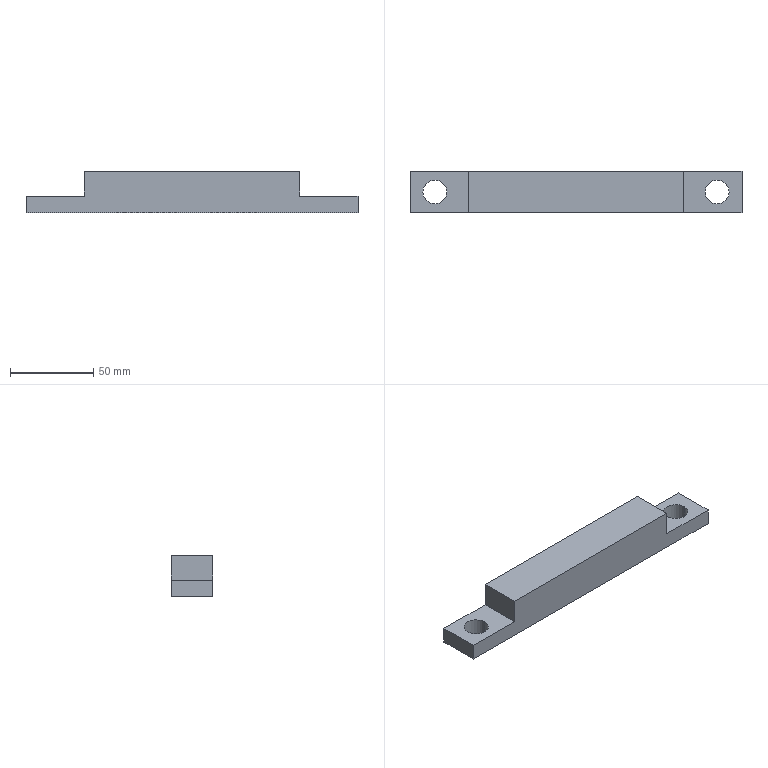Part | STEP file | 1 solid | 14 faces | box 200 x 25 x 25 mm | volume 95447 mm3 | plane 10 | cylinder 4 | commonest cylinder face diameters 14.5 x4
STEP:
#1=CARTESIAN_POINT('',(0.,0.,0.));
#2=DIRECTION('',(0.,0.,1.));
#3=DIRECTION('',(1.,0.,0.));
#4=AXIS2_PLACEMENT_3D('',#1,#2,#3);
#5=CARTESIAN_POINT('',(92.25,0.,0.));
#6=VERTEX_POINT('',#5);
#7=CARTESIAN_POINT('',(92.25,0.,10.));
#8=VERTEX_POINT('',#7);
#9=CARTESIAN_POINT('',(92.25,0.,-15.));
#10=DIRECTION('',(0.,0.,1.));
#11=VECTOR('',#10,1.);
#12=LINE('',#9,#11);
#13=CARTESIAN_POINT('',(85.,0.,-15.));
#14=DIRECTION('',(0.,0.,1.));
#15=DIRECTION('',(1.,0.,0.));
#16=AXIS2_PLACEMENT_3D('',#13,#14,#15);
#17=CYLINDRICAL_SURFACE('',#16,7.25);
#18=CARTESIAN_POINT('',(6.283,0.));
#19=DIRECTION('',(0.,1.));
#20=VECTOR('',#19,1.);
#21=LINE('',#18,#20);
#22=(GEOMETRIC_REPRESENTATION_CONTEXT(2)PARAMETRIC_REPRESENTATION_CONTEXT()REPRESENTATION_CONTEXT('',''));
#23=DEFINITIONAL_REPRESENTATION('',(#21),#22);
#24=PCURVE('',#17,#23);
#25=CARTESIAN_POINT('',(85.,0.,-15.));
#26=DIRECTION('',(0.,0.,1.));
#27=DIRECTION('',(1.,0.,0.));
#28=AXIS2_PLACEMENT_3D('',#25,#26,#27);
#29=CYLINDRICAL_SURFACE('',#28,7.25);
#30=CARTESIAN_POINT('',(0.,0.));
#31=DIRECTION('',(0.,1.));
#32=VECTOR('',#31,1.);
#33=LINE('',#30,#32);
#34=(GEOMETRIC_REPRESENTATION_CONTEXT(2)PARAMETRIC_REPRESENTATION_CONTEXT()REPRESENTATION_CONTEXT('',''));
#35=DEFINITIONAL_REPRESENTATION('',(#33),#34);
#36=PCURVE('',#29,#35);
#37=SURFACE_CURVE('',#12,(#24,#36),.PCURVE_S1.);
#38=EDGE_CURVE('',#6,#8,#37,.T.);
#39=ORIENTED_EDGE('',*,*,#38,.T.);
#40=CARTESIAN_POINT('',(77.75,0.,10.));
#41=VERTEX_POINT('',#40);
#42=CARTESIAN_POINT('',(85.,0.,10.));
#43=DIRECTION('',(0.,0.,1.));
#44=DIRECTION('',(1.,0.,0.));
#45=AXIS2_PLACEMENT_3D('',#42,#43,#44);
#46=CIRCLE('',#45,7.25);
#47=CARTESIAN_POINT('',(0.,25.));
#48=DIRECTION('',(1.,0.));
#49=VECTOR('',#48,1.);
#50=LINE('',#47,#49);
#51=(GEOMETRIC_REPRESENTATION_CONTEXT(2)PARAMETRIC_REPRESENTATION_CONTEXT()REPRESENTATION_CONTEXT('',''));
#52=DEFINITIONAL_REPRESENTATION('',(#50),#51);
#53=PCURVE('',#17,#52);
#54=CARTESIAN_POINT('',(100.,-12.5,10.));
#55=DIRECTION('',(0.,0.,-1.));
#56=DIRECTION('',(-1.,0.,0.));
#57=AXIS2_PLACEMENT_3D('',#54,#55,#56);
#58=PLANE('',#57);
#59=CARTESIAN_POINT('',(7.75,12.5));
#60=CARTESIAN_POINT('',(7.75,25.057));
#61=CARTESIAN_POINT('',(18.625,18.779));
#62=CARTESIAN_POINT('',(29.5,12.5));
#63=CARTESIAN_POINT('',(18.625,6.221));
#64=CARTESIAN_POINT('',(7.75,-0.05737));
#65=CARTESIAN_POINT('',(7.75,12.5));
#66=(BOUNDED_CURVE()B_SPLINE_CURVE(2,(#59,#60,#61,#62,#63,#64,#65),.UNSPECIFIED.,.T.,.F.)B_SPLINE_CURVE_WITH_KNOTS((1,2,2,2,2,1),(-2.094,0.,2.094,4.189,6.283,8.378),.UNSPECIFIED.)CURVE()GEOMETRIC_REPRESENTATION_ITEM()RATIONAL_B_SPLINE_CURVE((1.,0.5,1.,0.5,1.,0.5,1.))REPRESENTATION_ITEM(''));
#67=(GEOMETRIC_REPRESENTATION_CONTEXT(2)PARAMETRIC_REPRESENTATION_CONTEXT()REPRESENTATION_CONTEXT('',''));
#68=DEFINITIONAL_REPRESENTATION('',(#66),#67);
#69=PCURVE('',#58,#68);
#70=SURFACE_CURVE('',#46,(#53,#69),.PCURVE_S1.);
#71=EDGE_CURVE('',#41,#8,#70,.T.);
#72=ORIENTED_EDGE('',*,*,#71,.F.);
#73=CARTESIAN_POINT('',(77.75,0.,0.));
#74=VERTEX_POINT('',#73);
#75=CARTESIAN_POINT('',(77.75,0.,-15.));
#76=DIRECTION('',(0.,0.,1.));
#77=VECTOR('',#76,1.);
#78=LINE('',#75,#77);
#79=CARTESIAN_POINT('',(3.142,0.));
#80=DIRECTION('',(0.,1.));
#81=VECTOR('',#80,1.);
#82=LINE('',#79,#81);
#83=(GEOMETRIC_REPRESENTATION_CONTEXT(2)PARAMETRIC_REPRESENTATION_CONTEXT()REPRESENTATION_CONTEXT('',''));
#84=DEFINITIONAL_REPRESENTATION('',(#82),#83);
#85=PCURVE('',#17,#84);
#86=CARTESIAN_POINT('',(3.142,0.));
#87=DIRECTION('',(0.,1.));
#88=VECTOR('',#87,1.);
#89=LINE('',#86,#88);
#90=(GEOMETRIC_REPRESENTATION_CONTEXT(2)PARAMETRIC_REPRESENTATION_CONTEXT()REPRESENTATION_CONTEXT('',''));
#91=DEFINITIONAL_REPRESENTATION('',(#89),#90);
#92=PCURVE('',#29,#91);
#93=SURFACE_CURVE('',#78,(#85,#92),.PCURVE_S1.);
#94=EDGE_CURVE('',#74,#41,#93,.T.);
#95=ORIENTED_EDGE('',*,*,#94,.F.);
#96=CARTESIAN_POINT('',(85.,0.,0.));
#97=DIRECTION('',(0.,0.,-1.));
#98=DIRECTION('',(-1.,0.,0.));
#99=AXIS2_PLACEMENT_3D('',#96,#97,#98);
#100=CIRCLE('',#99,7.25);
#101=CARTESIAN_POINT('',(9.425,15.));
#102=DIRECTION('',(-1.,0.));
#103=VECTOR('',#102,1.);
#104=LINE('',#101,#103);
#105=(GEOMETRIC_REPRESENTATION_CONTEXT(2)PARAMETRIC_REPRESENTATION_CONTEXT()REPRESENTATION_CONTEXT('',''));
#106=DEFINITIONAL_REPRESENTATION('',(#104),#105);
#107=PCURVE('',#17,#106);
#108=CARTESIAN_POINT('',(0.,0.,0.));
#109=DIRECTION('',(0.,0.,-1.));
#110=DIRECTION('',(-1.,0.,0.));
#111=AXIS2_PLACEMENT_3D('',#108,#109,#110);
#112=PLANE('',#111);
#113=CARTESIAN_POINT('',(-85.,0.));
#114=DIRECTION('',(1.,0.));
#115=AXIS2_PLACEMENT_2D('',#113,#114);
#116=CIRCLE('',#115,7.25);
#117=(GEOMETRIC_REPRESENTATION_CONTEXT(2)PARAMETRIC_REPRESENTATION_CONTEXT()REPRESENTATION_CONTEXT('',''));
#118=DEFINITIONAL_REPRESENTATION('',(#116),#117);
#119=PCURVE('',#112,#118);
#120=SURFACE_CURVE('',#100,(#107,#119),.PCURVE_S1.);
#121=EDGE_CURVE('',#6,#74,#120,.T.);
#122=ORIENTED_EDGE('',*,*,#121,.F.);
#123=EDGE_LOOP('',(#39,#72,#95,#122));
#124=FACE_BOUND('',#123,.F.);
#125=ADVANCED_FACE('',(#124),#17,.F.);
#126=CARTESIAN_POINT('',(-77.75,0.,0.));
#127=VERTEX_POINT('',#126);
#128=CARTESIAN_POINT('',(-77.75,0.,10.));
#129=VERTEX_POINT('',#128);
#130=CARTESIAN_POINT('',(-77.75,0.,-15.));
#131=DIRECTION('',(0.,0.,1.));
#132=VECTOR('',#131,1.);
#133=LINE('',#130,#132);
#134=CARTESIAN_POINT('',(-85.,0.,-15.));
#135=DIRECTION('',(0.,0.,1.));
#136=DIRECTION('',(1.,0.,0.));
#137=AXIS2_PLACEMENT_3D('',#134,#135,#136);
#138=CYLINDRICAL_SURFACE('',#137,7.25);
#139=CARTESIAN_POINT('',(6.283,0.));
#140=DIRECTION('',(0.,1.));
#141=VECTOR('',#140,1.);
#142=LINE('',#139,#141);
#143=(GEOMETRIC_REPRESENTATION_CONTEXT(2)PARAMETRIC_REPRESENTATION_CONTEXT()REPRESENTATION_CONTEXT('',''));
#144=DEFINITIONAL_REPRESENTATION('',(#142),#143);
#145=PCURVE('',#138,#144);
#146=CARTESIAN_POINT('',(-85.,0.,-15.));
#147=DIRECTION('',(0.,0.,1.));
#148=DIRECTION('',(1.,0.,0.));
#149=AXIS2_PLACEMENT_3D('',#146,#147,#148);
#150=CYLINDRICAL_SURFACE('',#149,7.25);
#151=CARTESIAN_POINT('',(0.,0.));
#152=DIRECTION('',(0.,1.));
#153=VECTOR('',#152,1.);
#154=LINE('',#151,#153);
#155=(GEOMETRIC_REPRESENTATION_CONTEXT(2)PARAMETRIC_REPRESENTATION_CONTEXT()REPRESENTATION_CONTEXT('',''));
#156=DEFINITIONAL_REPRESENTATION('',(#154),#155);
#157=PCURVE('',#150,#156);
#158=SURFACE_CURVE('',#133,(#145,#157),.PCURVE_S1.);
#159=EDGE_CURVE('',#127,#129,#158,.T.);
#160=ORIENTED_EDGE('',*,*,#159,.T.);
#161=CARTESIAN_POINT('',(-92.25,0.,10.));
#162=VERTEX_POINT('',#161);
#163=CARTESIAN_POINT('',(-85.,0.,10.));
#164=DIRECTION('',(0.,0.,1.));
#165=DIRECTION('',(1.,0.,0.));
#166=AXIS2_PLACEMENT_3D('',#163,#164,#165);
#167=CIRCLE('',#166,7.25);
#168=CARTESIAN_POINT('',(0.,25.));
#169=DIRECTION('',(1.,0.));
#170=VECTOR('',#169,1.);
#171=LINE('',#168,#170);
#172=(GEOMETRIC_REPRESENTATION_CONTEXT(2)PARAMETRIC_REPRESENTATION_CONTEXT()REPRESENTATION_CONTEXT('',''));
#173=DEFINITIONAL_REPRESENTATION('',(#171),#172);
#174=PCURVE('',#138,#173);
#175=CARTESIAN_POINT('',(-100.,-12.5,10.));
#176=DIRECTION('',(0.,0.,-1.));
#177=DIRECTION('',(-1.,0.,0.));
#178=AXIS2_PLACEMENT_3D('',#175,#176,#177);
#179=PLANE('',#178);
#180=CARTESIAN_POINT('',(-22.25,12.5));
#181=CARTESIAN_POINT('',(-22.25,25.057));
#182=CARTESIAN_POINT('',(-11.375,18.779));
#183=CARTESIAN_POINT('',(-0.5,12.5));
#184=CARTESIAN_POINT('',(-11.375,6.221));
#185=CARTESIAN_POINT('',(-22.25,-0.05737));
#186=CARTESIAN_POINT('',(-22.25,12.5));
#187=(BOUNDED_CURVE()B_SPLINE_CURVE(2,(#180,#181,#182,#183,#184,#185,#186),.UNSPECIFIED.,.T.,.F.)B_SPLINE_CURVE_WITH_KNOTS((1,2,2,2,2,1),(-2.094,0.,2.094,4.189,6.283,8.378),.UNSPECIFIED.)CURVE()GEOMETRIC_REPRESENTATION_ITEM()RATIONAL_B_SPLINE_CURVE((1.,0.5,1.,0.5,1.,0.5,1.))REPRESENTATION_ITEM(''));
#188=(GEOMETRIC_REPRESENTATION_CONTEXT(2)PARAMETRIC_REPRESENTATION_CONTEXT()REPRESENTATION_CONTEXT('',''));
#189=DEFINITIONAL_REPRESENTATION('',(#187),#188);
#190=PCURVE('',#179,#189);
#191=SURFACE_CURVE('',#167,(#174,#190),.PCURVE_S1.);
#192=EDGE_CURVE('',#162,#129,#191,.T.);
#193=ORIENTED_EDGE('',*,*,#192,.F.);
#194=CARTESIAN_POINT('',(-92.25,0.,0.));
#195=VERTEX_POINT('',#194);
#196=CARTESIAN_POINT('',(-92.25,0.,-15.));
#197=DIRECTION('',(0.,0.,1.));
#198=VECTOR('',#197,1.);
#199=LINE('',#196,#198);
#200=CARTESIAN_POINT('',(3.142,0.));
#201=DIRECTION('',(0.,1.));
#202=VECTOR('',#201,1.);
#203=LINE('',#200,#202);
#204=(GEOMETRIC_REPRESENTATION_CONTEXT(2)PARAMETRIC_REPRESENTATION_CONTEXT()REPRESENTATION_CONTEXT('',''));
#205=DEFINITIONAL_REPRESENTATION('',(#203),#204);
#206=PCURVE('',#138,#205);
#207=CARTESIAN_POINT('',(3.142,0.));
#208=DIRECTION('',(0.,1.));
#209=VECTOR('',#208,1.);
#210=LINE('',#207,#209);
#211=(GEOMETRIC_REPRESENTATION_CONTEXT(2)PARAMETRIC_REPRESENTATION_CONTEXT()REPRESENTATION_CONTEXT('',''));
#212=DEFINITIONAL_REPRESENTATION('',(#210),#211);
#213=PCURVE('',#150,#212);
#214=SURFACE_CURVE('',#199,(#206,#213),.PCURVE_S1.);
#215=EDGE_CURVE('',#195,#162,#214,.T.);
#216=ORIENTED_EDGE('',*,*,#215,.F.);
#217=CARTESIAN_POINT('',(-85.,0.,0.));
#218=DIRECTION('',(0.,0.,-1.));
#219=DIRECTION('',(-1.,0.,0.));
#220=AXIS2_PLACEMENT_3D('',#217,#218,#219);
#221=CIRCLE('',#220,7.25);
#222=CARTESIAN_POINT('',(9.425,15.));
#223=DIRECTION('',(-1.,0.));
#224=VECTOR('',#223,1.);
#225=LINE('',#222,#224);
#226=(GEOMETRIC_REPRESENTATION_CONTEXT(2)PARAMETRIC_REPRESENTATION_CONTEXT()REPRESENTATION_CONTEXT('',''));
#227=DEFINITIONAL_REPRESENTATION('',(#225),#226);
#228=PCURVE('',#138,#227);
#229=CARTESIAN_POINT('',(85.,0.));
#230=DIRECTION('',(1.,0.));
#231=AXIS2_PLACEMENT_2D('',#229,#230);
#232=CIRCLE('',#231,7.25);
#233=(GEOMETRIC_REPRESENTATION_CONTEXT(2)PARAMETRIC_REPRESENTATION_CONTEXT()REPRESENTATION_CONTEXT('',''));
#234=DEFINITIONAL_REPRESENTATION('',(#232),#233);
#235=PCURVE('',#112,#234);
#236=SURFACE_CURVE('',#221,(#228,#235),.PCURVE_S1.);
#237=EDGE_CURVE('',#127,#195,#236,.T.);
#238=ORIENTED_EDGE('',*,*,#237,.F.);
#239=EDGE_LOOP('',(#160,#193,#216,#238));
#240=FACE_BOUND('',#239,.F.);
#241=ADVANCED_FACE('',(#240),#138,.F.);
#242=CARTESIAN_POINT('',(-100.,-12.5,10.));
#243=VERTEX_POINT('',#242);
#244=CARTESIAN_POINT('',(-100.,-12.5,0.));
#245=VERTEX_POINT('',#244);
#246=CARTESIAN_POINT('',(-100.,-12.5,25.));
#247=DIRECTION('',(0.,0.,-1.));
#248=VECTOR('',#247,1.);
#249=LINE('',#246,#248);
#250=CARTESIAN_POINT('',(-100.,12.5,25.));
#251=DIRECTION('',(1.,0.,0.));
#252=DIRECTION('',(0.,0.,-1.));
#253=AXIS2_PLACEMENT_3D('',#250,#251,#252);
#254=PLANE('',#253);
#255=CARTESIAN_POINT('',(0.,-25.));
#256=DIRECTION('',(1.,0.));
#257=VECTOR('',#256,1.);
#258=LINE('',#255,#257);
#259=(GEOMETRIC_REPRESENTATION_CONTEXT(2)PARAMETRIC_REPRESENTATION_CONTEXT()REPRESENTATION_CONTEXT('',''));
#260=DEFINITIONAL_REPRESENTATION('',(#258),#259);
#261=PCURVE('',#254,#260);
#262=CARTESIAN_POINT('',(100.,-12.5,25.));
#263=DIRECTION('',(0.,1.,0.));
#264=DIRECTION('',(-1.,0.,0.));
#265=AXIS2_PLACEMENT_3D('',#262,#263,#264);
#266=PLANE('',#265);
#267=CARTESIAN_POINT('',(200.,0.));
#268=DIRECTION('',(0.,-1.));
#269=VECTOR('',#268,1.);
#270=LINE('',#267,#269);
#271=(GEOMETRIC_REPRESENTATION_CONTEXT(2)PARAMETRIC_REPRESENTATION_CONTEXT()REPRESENTATION_CONTEXT('',''));
#272=DEFINITIONAL_REPRESENTATION('',(#270),#271);
#273=PCURVE('',#266,#272);
#274=SURFACE_CURVE('',#249,(#261,#273),.PCURVE_S1.);
#275=EDGE_CURVE('',#243,#245,#274,.T.);
#276=ORIENTED_EDGE('',*,*,#275,.F.);
#277=CARTESIAN_POINT('',(-100.,12.5,10.));
#278=VERTEX_POINT('',#277);
#279=CARTESIAN_POINT('',(-100.,-12.5,10.));
#280=DIRECTION('',(0.,1.,0.));
#281=VECTOR('',#280,1.);
#282=LINE('',#279,#281);
#283=CARTESIAN_POINT('',(15.,-25.));
#284=DIRECTION('',(0.,1.));
#285=VECTOR('',#284,1.);
#286=LINE('',#283,#285);
#287=(GEOMETRIC_REPRESENTATION_CONTEXT(2)PARAMETRIC_REPRESENTATION_CONTEXT()REPRESENTATION_CONTEXT('',''));
#288=DEFINITIONAL_REPRESENTATION('',(#286),#287);
#289=PCURVE('',#254,#288);
#290=CARTESIAN_POINT('',(0.,0.));
#291=DIRECTION('',(0.,1.));
#292=VECTOR('',#291,1.);
#293=LINE('',#290,#292);
#294=(GEOMETRIC_REPRESENTATION_CONTEXT(2)PARAMETRIC_REPRESENTATION_CONTEXT()REPRESENTATION_CONTEXT('',''));
#295=DEFINITIONAL_REPRESENTATION('',(#293),#294);
#296=PCURVE('',#179,#295);
#297=SURFACE_CURVE('',#282,(#289,#296),.PCURVE_S1.);
#298=EDGE_CURVE('',#243,#278,#297,.T.);
#299=ORIENTED_EDGE('',*,*,#298,.T.);
#300=CARTESIAN_POINT('',(-100.,12.5,0.));
#301=VERTEX_POINT('',#300);
#302=CARTESIAN_POINT('',(-100.,12.5,25.));
#303=DIRECTION('',(0.,0.,-1.));
#304=VECTOR('',#303,1.);
#305=LINE('',#302,#304);
#306=CARTESIAN_POINT('',(0.,0.));
#307=DIRECTION('',(1.,0.));
#308=VECTOR('',#307,1.);
#309=LINE('',#306,#308);
#310=(GEOMETRIC_REPRESENTATION_CONTEXT(2)PARAMETRIC_REPRESENTATION_CONTEXT()REPRESENTATION_CONTEXT('',''));
#311=DEFINITIONAL_REPRESENTATION('',(#309),#310);
#312=PCURVE('',#254,#311);
#313=CARTESIAN_POINT('',(100.,12.5,25.));
#314=DIRECTION('',(0.,-1.,0.));
#315=DIRECTION('',(1.,0.,0.));
#316=AXIS2_PLACEMENT_3D('',#313,#314,#315);
#317=PLANE('',#316);
#318=CARTESIAN_POINT('',(-200.,0.));
#319=DIRECTION('',(0.,-1.));
#320=VECTOR('',#319,1.);
#321=LINE('',#318,#320);
#322=(GEOMETRIC_REPRESENTATION_CONTEXT(2)PARAMETRIC_REPRESENTATION_CONTEXT()REPRESENTATION_CONTEXT('',''));
#323=DEFINITIONAL_REPRESENTATION('',(#321),#322);
#324=PCURVE('',#317,#323);
#325=SURFACE_CURVE('',#305,(#312,#324),.PCURVE_S1.);
#326=EDGE_CURVE('',#278,#301,#325,.T.);
#327=ORIENTED_EDGE('',*,*,#326,.T.);
#328=CARTESIAN_POINT('',(-100.,12.5,0.));
#329=DIRECTION('',(0.,-1.,0.));
#330=VECTOR('',#329,1.);
#331=LINE('',#328,#330);
#332=CARTESIAN_POINT('',(25.,0.));
#333=DIRECTION('',(0.,-1.));
#334=VECTOR('',#333,1.);
#335=LINE('',#332,#334);
#336=(GEOMETRIC_REPRESENTATION_CONTEXT(2)PARAMETRIC_REPRESENTATION_CONTEXT()REPRESENTATION_CONTEXT('',''));
#337=DEFINITIONAL_REPRESENTATION('',(#335),#336);
#338=PCURVE('',#254,#337);
#339=CARTESIAN_POINT('',(100.,12.5));
#340=DIRECTION('',(0.,-1.));
#341=VECTOR('',#340,1.);
#342=LINE('',#339,#341);
#343=(GEOMETRIC_REPRESENTATION_CONTEXT(2)PARAMETRIC_REPRESENTATION_CONTEXT()REPRESENTATION_CONTEXT('',''));
#344=DEFINITIONAL_REPRESENTATION('',(#342),#343);
#345=PCURVE('',#112,#344);
#346=SURFACE_CURVE('',#331,(#338,#345),.PCURVE_S1.);
#347=EDGE_CURVE('',#301,#245,#346,.T.);
#348=ORIENTED_EDGE('',*,*,#347,.T.);
#349=EDGE_LOOP('',(#276,#299,#327,#348));
#350=FACE_BOUND('',#349,.T.);
#351=ADVANCED_FACE('',(#350),#254,.F.);
#352=CARTESIAN_POINT('',(-65.,-12.5,25.));
#353=VERTEX_POINT('',#352);
#354=CARTESIAN_POINT('',(-65.,-12.5,10.));
#355=VERTEX_POINT('',#354);
#356=CARTESIAN_POINT('',(-65.,-12.5,10.));
#357=DIRECTION('',(0.,0.,-1.));
#358=VECTOR('',#357,1.);
#359=LINE('',#356,#358);
#360=CARTESIAN_POINT('',(165.,-15.));
#361=DIRECTION('',(0.,-1.));
#362=VECTOR('',#361,1.);
#363=LINE('',#360,#362);
#364=(GEOMETRIC_REPRESENTATION_CONTEXT(2)PARAMETRIC_REPRESENTATION_CONTEXT()REPRESENTATION_CONTEXT('',''));
#365=DEFINITIONAL_REPRESENTATION('',(#363),#364);
#366=PCURVE('',#266,#365);
#367=CARTESIAN_POINT('',(-65.,-12.5,10.));
#368=DIRECTION('',(1.,0.,0.));
#369=DIRECTION('',(0.,1.,0.));
#370=AXIS2_PLACEMENT_3D('',#367,#368,#369);
#371=PLANE('',#370);
#372=CARTESIAN_POINT('',(0.,0.));
#373=DIRECTION('',(0.,-1.));
#374=VECTOR('',#373,1.);
#375=LINE('',#372,#374);
#376=(GEOMETRIC_REPRESENTATION_CONTEXT(2)PARAMETRIC_REPRESENTATION_CONTEXT()REPRESENTATION_CONTEXT('',''));
#377=DEFINITIONAL_REPRESENTATION('',(#375),#376);
#378=PCURVE('',#371,#377);
#379=SURFACE_CURVE('',#359,(#366,#378),.PCURVE_S1.);
#380=EDGE_CURVE('',#353,#355,#379,.T.);
#381=ORIENTED_EDGE('',*,*,#380,.T.);
#382=CARTESIAN_POINT('',(-100.,-12.5,10.));
#383=DIRECTION('',(-1.,0.,0.));
#384=VECTOR('',#383,1.);
#385=LINE('',#382,#384);
#386=CARTESIAN_POINT('',(200.,-15.));
#387=DIRECTION('',(1.,0.));
#388=VECTOR('',#387,1.);
#389=LINE('',#386,#388);
#390=(GEOMETRIC_REPRESENTATION_CONTEXT(2)PARAMETRIC_REPRESENTATION_CONTEXT()REPRESENTATION_CONTEXT('',''));
#391=DEFINITIONAL_REPRESENTATION('',(#389),#390);
#392=PCURVE('',#266,#391);
#393=CARTESIAN_POINT('',(0.,0.));
#394=DIRECTION('',(1.,0.));
#395=VECTOR('',#394,1.);
#396=LINE('',#393,#395);
#397=(GEOMETRIC_REPRESENTATION_CONTEXT(2)PARAMETRIC_REPRESENTATION_CONTEXT()REPRESENTATION_CONTEXT('',''));
#398=DEFINITIONAL_REPRESENTATION('',(#396),#397);
#399=PCURVE('',#179,#398);
#400=SURFACE_CURVE('',#385,(#392,#399),.PCURVE_S1.);
#401=EDGE_CURVE('',#355,#243,#400,.T.);
#402=ORIENTED_EDGE('',*,*,#401,.T.);
#403=ORIENTED_EDGE('',*,*,#275,.T.);
#404=CARTESIAN_POINT('',(100.,-12.5,0.));
#405=VERTEX_POINT('',#404);
#406=CARTESIAN_POINT('',(100.,-12.5,0.));
#407=DIRECTION('',(1.,0.,0.));
#408=VECTOR('',#407,1.);
#409=LINE('',#406,#408);
#410=CARTESIAN_POINT('',(0.,-25.));
#411=DIRECTION('',(-1.,0.));
#412=VECTOR('',#411,1.);
#413=LINE('',#410,#412);
#414=(GEOMETRIC_REPRESENTATION_CONTEXT(2)PARAMETRIC_REPRESENTATION_CONTEXT()REPRESENTATION_CONTEXT('',''));
#415=DEFINITIONAL_REPRESENTATION('',(#413),#414);
#416=PCURVE('',#266,#415);
#417=CARTESIAN_POINT('',(-100.,-12.5));
#418=DIRECTION('',(-1.,0.));
#419=VECTOR('',#418,1.);
#420=LINE('',#417,#419);
#421=(GEOMETRIC_REPRESENTATION_CONTEXT(2)PARAMETRIC_REPRESENTATION_CONTEXT()REPRESENTATION_CONTEXT('',''));
#422=DEFINITIONAL_REPRESENTATION('',(#420),#421);
#423=PCURVE('',#112,#422);
#424=SURFACE_CURVE('',#409,(#416,#423),.PCURVE_S1.);
#425=EDGE_CURVE('',#245,#405,#424,.T.);
#426=ORIENTED_EDGE('',*,*,#425,.T.);
#427=CARTESIAN_POINT('',(100.,-12.5,10.));
#428=VERTEX_POINT('',#427);
#429=CARTESIAN_POINT('',(100.,-12.5,25.));
#430=DIRECTION('',(0.,0.,-1.));
#431=VECTOR('',#430,1.);
#432=LINE('',#429,#431);
#433=CARTESIAN_POINT('',(0.,0.));
#434=DIRECTION('',(0.,-1.));
#435=VECTOR('',#434,1.);
#436=LINE('',#433,#435);
#437=(GEOMETRIC_REPRESENTATION_CONTEXT(2)PARAMETRIC_REPRESENTATION_CONTEXT()REPRESENTATION_CONTEXT('',''));
#438=DEFINITIONAL_REPRESENTATION('',(#436),#437);
#439=PCURVE('',#266,#438);
#440=CARTESIAN_POINT('',(100.,12.5,25.));
#441=DIRECTION('',(-1.,0.,0.));
#442=DIRECTION('',(0.,0.,1.));
#443=AXIS2_PLACEMENT_3D('',#440,#441,#442);
#444=PLANE('',#443);
#445=CARTESIAN_POINT('',(0.,-25.));
#446=DIRECTION('',(-1.,0.));
#447=VECTOR('',#446,1.);
#448=LINE('',#445,#447);
#449=(GEOMETRIC_REPRESENTATION_CONTEXT(2)PARAMETRIC_REPRESENTATION_CONTEXT()REPRESENTATION_CONTEXT('',''));
#450=DEFINITIONAL_REPRESENTATION('',(#448),#449);
#451=PCURVE('',#444,#450);
#452=SURFACE_CURVE('',#432,(#439,#451),.PCURVE_S1.);
#453=EDGE_CURVE('',#428,#405,#452,.T.);
#454=ORIENTED_EDGE('',*,*,#453,.F.);
#455=CARTESIAN_POINT('',(65.,-12.5,10.));
#456=VERTEX_POINT('',#455);
#457=CARTESIAN_POINT('',(100.,-12.5,10.));
#458=DIRECTION('',(-1.,0.,0.));
#459=VECTOR('',#458,1.);
#460=LINE('',#457,#459);
#461=CARTESIAN_POINT('',(0.,-15.));
#462=DIRECTION('',(1.,0.));
#463=VECTOR('',#462,1.);
#464=LINE('',#461,#463);
#465=(GEOMETRIC_REPRESENTATION_CONTEXT(2)PARAMETRIC_REPRESENTATION_CONTEXT()REPRESENTATION_CONTEXT('',''));
#466=DEFINITIONAL_REPRESENTATION('',(#464),#465);
#467=PCURVE('',#266,#466);
#468=CARTESIAN_POINT('',(0.,0.));
#469=DIRECTION('',(1.,0.));
#470=VECTOR('',#469,1.);
#471=LINE('',#468,#470);
#472=(GEOMETRIC_REPRESENTATION_CONTEXT(2)PARAMETRIC_REPRESENTATION_CONTEXT()REPRESENTATION_CONTEXT('',''));
#473=DEFINITIONAL_REPRESENTATION('',(#471),#472);
#474=PCURVE('',#58,#473);
#475=SURFACE_CURVE('',#460,(#467,#474),.PCURVE_S1.);
#476=EDGE_CURVE('',#428,#456,#475,.T.);
#477=ORIENTED_EDGE('',*,*,#476,.T.);
#478=CARTESIAN_POINT('',(65.,-12.5,25.));
#479=VERTEX_POINT('',#478);
#480=CARTESIAN_POINT('',(65.,-12.5,10.));
#481=DIRECTION('',(0.,0.,1.));
#482=VECTOR('',#481,1.);
#483=LINE('',#480,#482);
#484=CARTESIAN_POINT('',(35.,-15.));
#485=DIRECTION('',(0.,1.));
#486=VECTOR('',#485,1.);
#487=LINE('',#484,#486);
#488=(GEOMETRIC_REPRESENTATION_CONTEXT(2)PARAMETRIC_REPRESENTATION_CONTEXT()REPRESENTATION_CONTEXT('',''));
#489=DEFINITIONAL_REPRESENTATION('',(#487),#488);
#490=PCURVE('',#266,#489);
#491=CARTESIAN_POINT('',(65.,-12.5,10.));
#492=DIRECTION('',(-1.,0.,0.));
#493=DIRECTION('',(0.,-1.,0.));
#494=AXIS2_PLACEMENT_3D('',#491,#492,#493);
#495=PLANE('',#494);
#496=CARTESIAN_POINT('',(0.,0.));
#497=DIRECTION('',(0.,1.));
#498=VECTOR('',#497,1.);
#499=LINE('',#496,#498);
#500=(GEOMETRIC_REPRESENTATION_CONTEXT(2)PARAMETRIC_REPRESENTATION_CONTEXT()REPRESENTATION_CONTEXT('',''));
#501=DEFINITIONAL_REPRESENTATION('',(#499),#500);
#502=PCURVE('',#495,#501);
#503=SURFACE_CURVE('',#483,(#490,#502),.PCURVE_S1.);
#504=EDGE_CURVE('',#456,#479,#503,.T.);
#505=ORIENTED_EDGE('',*,*,#504,.T.);
#506=CARTESIAN_POINT('',(100.,-12.5,25.));
#507=DIRECTION('',(1.,0.,0.));
#508=VECTOR('',#507,1.);
#509=LINE('',#506,#508);
#510=CARTESIAN_POINT('',(0.,0.));
#511=DIRECTION('',(-1.,0.));
#512=VECTOR('',#511,1.);
#513=LINE('',#510,#512);
#514=(GEOMETRIC_REPRESENTATION_CONTEXT(2)PARAMETRIC_REPRESENTATION_CONTEXT()REPRESENTATION_CONTEXT('',''));
#515=DEFINITIONAL_REPRESENTATION('',(#513),#514);
#516=PCURVE('',#266,#515);
#517=CARTESIAN_POINT('',(0.,0.,25.));
#518=DIRECTION('',(0.,0.,-1.));
#519=DIRECTION('',(-1.,0.,0.));
#520=AXIS2_PLACEMENT_3D('',#517,#518,#519);
#521=PLANE('',#520);
#522=CARTESIAN_POINT('',(-100.,-12.5));
#523=DIRECTION('',(-1.,0.));
#524=VECTOR('',#523,1.);
#525=LINE('',#522,#524);
#526=(GEOMETRIC_REPRESENTATION_CONTEXT(2)PARAMETRIC_REPRESENTATION_CONTEXT()REPRESENTATION_CONTEXT('',''));
#527=DEFINITIONAL_REPRESENTATION('',(#525),#526);
#528=PCURVE('',#521,#527);
#529=SURFACE_CURVE('',#509,(#516,#528),.PCURVE_S1.);
#530=EDGE_CURVE('',#353,#479,#529,.T.);
#531=ORIENTED_EDGE('',*,*,#530,.F.);
#532=EDGE_LOOP('',(#381,#402,#403,#426,#454,#477,#505,#531));
#533=FACE_BOUND('',#532,.T.);
#534=ADVANCED_FACE('',(#533),#266,.F.);
#535=CARTESIAN_POINT('',(100.,12.5,10.));
#536=VERTEX_POINT('',#535);
#537=CARTESIAN_POINT('',(100.,12.5,0.));
#538=VERTEX_POINT('',#537);
#539=CARTESIAN_POINT('',(100.,12.5,25.));
#540=DIRECTION('',(0.,0.,-1.));
#541=VECTOR('',#540,1.);
#542=LINE('',#539,#541);
#543=CARTESIAN_POINT('',(0.,0.));
#544=DIRECTION('',(-1.,0.));
#545=VECTOR('',#544,1.);
#546=LINE('',#543,#545);
#547=(GEOMETRIC_REPRESENTATION_CONTEXT(2)PARAMETRIC_REPRESENTATION_CONTEXT()REPRESENTATION_CONTEXT('',''));
#548=DEFINITIONAL_REPRESENTATION('',(#546),#547);
#549=PCURVE('',#444,#548);
#550=CARTESIAN_POINT('',(0.,0.));
#551=DIRECTION('',(0.,-1.));
#552=VECTOR('',#551,1.);
#553=LINE('',#550,#552);
#554=(GEOMETRIC_REPRESENTATION_CONTEXT(2)PARAMETRIC_REPRESENTATION_CONTEXT()REPRESENTATION_CONTEXT('',''));
#555=DEFINITIONAL_REPRESENTATION('',(#553),#554);
#556=PCURVE('',#317,#555);
#557=SURFACE_CURVE('',#542,(#549,#556),.PCURVE_S1.);
#558=EDGE_CURVE('',#536,#538,#557,.T.);
#559=ORIENTED_EDGE('',*,*,#558,.F.);
#560=CARTESIAN_POINT('',(100.,-12.5,10.));
#561=DIRECTION('',(0.,1.,0.));
#562=VECTOR('',#561,1.);
#563=LINE('',#560,#562);
#564=CARTESIAN_POINT('',(-15.,-25.));
#565=DIRECTION('',(0.,1.));
#566=VECTOR('',#565,1.);
#567=LINE('',#564,#566);
#568=(GEOMETRIC_REPRESENTATION_CONTEXT(2)PARAMETRIC_REPRESENTATION_CONTEXT()REPRESENTATION_CONTEXT('',''));
#569=DEFINITIONAL_REPRESENTATION('',(#567),#568);
#570=PCURVE('',#444,#569);
#571=CARTESIAN_POINT('',(0.,0.));
#572=DIRECTION('',(0.,1.));
#573=VECTOR('',#572,1.);
#574=LINE('',#571,#573);
#575=(GEOMETRIC_REPRESENTATION_CONTEXT(2)PARAMETRIC_REPRESENTATION_CONTEXT()REPRESENTATION_CONTEXT('',''));
#576=DEFINITIONAL_REPRESENTATION('',(#574),#575);
#577=PCURVE('',#58,#576);
#578=SURFACE_CURVE('',#563,(#570,#577),.PCURVE_S1.);
#579=EDGE_CURVE('',#428,#536,#578,.T.);
#580=ORIENTED_EDGE('',*,*,#579,.F.);
#581=ORIENTED_EDGE('',*,*,#453,.T.);
#582=CARTESIAN_POINT('',(100.,12.5,0.));
#583=DIRECTION('',(0.,1.,0.));
#584=VECTOR('',#583,1.);
#585=LINE('',#582,#584);
#586=CARTESIAN_POINT('',(-25.,0.));
#587=DIRECTION('',(0.,1.));
#588=VECTOR('',#587,1.);
#589=LINE('',#586,#588);
#590=(GEOMETRIC_REPRESENTATION_CONTEXT(2)PARAMETRIC_REPRESENTATION_CONTEXT()REPRESENTATION_CONTEXT('',''));
#591=DEFINITIONAL_REPRESENTATION('',(#589),#590);
#592=PCURVE('',#444,#591);
#593=CARTESIAN_POINT('',(-100.,12.5));
#594=DIRECTION('',(0.,1.));
#595=VECTOR('',#594,1.);
#596=LINE('',#593,#595);
#597=(GEOMETRIC_REPRESENTATION_CONTEXT(2)PARAMETRIC_REPRESENTATION_CONTEXT()REPRESENTATION_CONTEXT('',''));
#598=DEFINITIONAL_REPRESENTATION('',(#596),#597);
#599=PCURVE('',#112,#598);
#600=SURFACE_CURVE('',#585,(#592,#599),.PCURVE_S1.);
#601=EDGE_CURVE('',#405,#538,#600,.T.);
#602=ORIENTED_EDGE('',*,*,#601,.T.);
#603=EDGE_LOOP('',(#559,#580,#581,#602));
#604=FACE_BOUND('',#603,.T.);
#605=ADVANCED_FACE('',(#604),#444,.F.);
#606=ORIENTED_EDGE('',*,*,#326,.F.);
#607=CARTESIAN_POINT('',(-65.,12.5,10.));
#608=VERTEX_POINT('',#607);
#609=CARTESIAN_POINT('',(-100.,12.5,10.));
#610=DIRECTION('',(-1.,0.,0.));
#611=VECTOR('',#610,1.);
#612=LINE('',#609,#611);
#613=CARTESIAN_POINT('',(-200.,-15.));
#614=DIRECTION('',(-1.,0.));
#615=VECTOR('',#614,1.);
#616=LINE('',#613,#615);
#617=(GEOMETRIC_REPRESENTATION_CONTEXT(2)PARAMETRIC_REPRESENTATION_CONTEXT()REPRESENTATION_CONTEXT('',''));
#618=DEFINITIONAL_REPRESENTATION('',(#616),#617);
#619=PCURVE('',#317,#618);
#620=CARTESIAN_POINT('',(0.,25.));
#621=DIRECTION('',(1.,0.));
#622=VECTOR('',#621,1.);
#623=LINE('',#620,#622);
#624=(GEOMETRIC_REPRESENTATION_CONTEXT(2)PARAMETRIC_REPRESENTATION_CONTEXT()REPRESENTATION_CONTEXT('',''));
#625=DEFINITIONAL_REPRESENTATION('',(#623),#624);
#626=PCURVE('',#179,#625);
#627=SURFACE_CURVE('',#612,(#619,#626),.PCURVE_S1.);
#628=EDGE_CURVE('',#608,#278,#627,.T.);
#629=ORIENTED_EDGE('',*,*,#628,.F.);
#630=CARTESIAN_POINT('',(-65.,12.5,25.));
#631=VERTEX_POINT('',#630);
#632=CARTESIAN_POINT('',(-65.,12.5,10.));
#633=DIRECTION('',(0.,0.,-1.));
#634=VECTOR('',#633,1.);
#635=LINE('',#632,#634);
#636=CARTESIAN_POINT('',(-165.,-15.));
#637=DIRECTION('',(0.,-1.));
#638=VECTOR('',#637,1.);
#639=LINE('',#636,#638);
#640=(GEOMETRIC_REPRESENTATION_CONTEXT(2)PARAMETRIC_REPRESENTATION_CONTEXT()REPRESENTATION_CONTEXT('',''));
#641=DEFINITIONAL_REPRESENTATION('',(#639),#640);
#642=PCURVE('',#317,#641);
#643=CARTESIAN_POINT('',(25.,0.));
#644=DIRECTION('',(0.,-1.));
#645=VECTOR('',#644,1.);
#646=LINE('',#643,#645);
#647=(GEOMETRIC_REPRESENTATION_CONTEXT(2)PARAMETRIC_REPRESENTATION_CONTEXT()REPRESENTATION_CONTEXT('',''));
#648=DEFINITIONAL_REPRESENTATION('',(#646),#647);
#649=PCURVE('',#371,#648);
#650=SURFACE_CURVE('',#635,(#642,#649),.PCURVE_S1.);
#651=EDGE_CURVE('',#631,#608,#650,.T.);
#652=ORIENTED_EDGE('',*,*,#651,.F.);
#653=CARTESIAN_POINT('',(65.,12.5,25.));
#654=VERTEX_POINT('',#653);
#655=CARTESIAN_POINT('',(100.,12.5,25.));
#656=DIRECTION('',(-1.,0.,0.));
#657=VECTOR('',#656,1.);
#658=LINE('',#655,#657);
#659=CARTESIAN_POINT('',(0.,0.));
#660=DIRECTION('',(-1.,0.));
#661=VECTOR('',#660,1.);
#662=LINE('',#659,#661);
#663=(GEOMETRIC_REPRESENTATION_CONTEXT(2)PARAMETRIC_REPRESENTATION_CONTEXT()REPRESENTATION_CONTEXT('',''));
#664=DEFINITIONAL_REPRESENTATION('',(#662),#663);
#665=PCURVE('',#317,#664);
#666=CARTESIAN_POINT('',(-100.,12.5));
#667=DIRECTION('',(1.,0.));
#668=VECTOR('',#667,1.);
#669=LINE('',#666,#668);
#670=(GEOMETRIC_REPRESENTATION_CONTEXT(2)PARAMETRIC_REPRESENTATION_CONTEXT()REPRESENTATION_CONTEXT('',''));
#671=DEFINITIONAL_REPRESENTATION('',(#669),#670);
#672=PCURVE('',#521,#671);
#673=SURFACE_CURVE('',#658,(#665,#672),.PCURVE_S1.);
#674=EDGE_CURVE('',#654,#631,#673,.T.);
#675=ORIENTED_EDGE('',*,*,#674,.F.);
#676=CARTESIAN_POINT('',(65.,12.5,10.));
#677=VERTEX_POINT('',#676);
#678=CARTESIAN_POINT('',(65.,12.5,10.));
#679=DIRECTION('',(0.,0.,1.));
#680=VECTOR('',#679,1.);
#681=LINE('',#678,#680);
#682=CARTESIAN_POINT('',(-35.,-15.));
#683=DIRECTION('',(0.,1.));
#684=VECTOR('',#683,1.);
#685=LINE('',#682,#684);
#686=(GEOMETRIC_REPRESENTATION_CONTEXT(2)PARAMETRIC_REPRESENTATION_CONTEXT()REPRESENTATION_CONTEXT('',''));
#687=DEFINITIONAL_REPRESENTATION('',(#685),#686);
#688=PCURVE('',#317,#687);
#689=CARTESIAN_POINT('',(-25.,0.));
#690=DIRECTION('',(0.,1.));
#691=VECTOR('',#690,1.);
#692=LINE('',#689,#691);
#693=(GEOMETRIC_REPRESENTATION_CONTEXT(2)PARAMETRIC_REPRESENTATION_CONTEXT()REPRESENTATION_CONTEXT('',''));
#694=DEFINITIONAL_REPRESENTATION('',(#692),#693);
#695=PCURVE('',#495,#694);
#696=SURFACE_CURVE('',#681,(#688,#695),.PCURVE_S1.);
#697=EDGE_CURVE('',#677,#654,#696,.T.);
#698=ORIENTED_EDGE('',*,*,#697,.F.);
#699=CARTESIAN_POINT('',(100.,12.5,10.));
#700=DIRECTION('',(-1.,0.,0.));
#701=VECTOR('',#700,1.);
#702=LINE('',#699,#701);
#703=CARTESIAN_POINT('',(0.,-15.));
#704=DIRECTION('',(-1.,0.));
#705=VECTOR('',#704,1.);
#706=LINE('',#703,#705);
#707=(GEOMETRIC_REPRESENTATION_CONTEXT(2)PARAMETRIC_REPRESENTATION_CONTEXT()REPRESENTATION_CONTEXT('',''));
#708=DEFINITIONAL_REPRESENTATION('',(#706),#707);
#709=PCURVE('',#317,#708);
#710=CARTESIAN_POINT('',(0.,25.));
#711=DIRECTION('',(1.,0.));
#712=VECTOR('',#711,1.);
#713=LINE('',#710,#712);
#714=(GEOMETRIC_REPRESENTATION_CONTEXT(2)PARAMETRIC_REPRESENTATION_CONTEXT()REPRESENTATION_CONTEXT('',''));
#715=DEFINITIONAL_REPRESENTATION('',(#713),#714);
#716=PCURVE('',#58,#715);
#717=SURFACE_CURVE('',#702,(#709,#716),.PCURVE_S1.);
#718=EDGE_CURVE('',#536,#677,#717,.T.);
#719=ORIENTED_EDGE('',*,*,#718,.F.);
#720=ORIENTED_EDGE('',*,*,#558,.T.);
#721=CARTESIAN_POINT('',(100.,12.5,0.));
#722=DIRECTION('',(-1.,0.,0.));
#723=VECTOR('',#722,1.);
#724=LINE('',#721,#723);
#725=CARTESIAN_POINT('',(0.,-25.));
#726=DIRECTION('',(-1.,0.));
#727=VECTOR('',#726,1.);
#728=LINE('',#725,#727);
#729=(GEOMETRIC_REPRESENTATION_CONTEXT(2)PARAMETRIC_REPRESENTATION_CONTEXT()REPRESENTATION_CONTEXT('',''));
#730=DEFINITIONAL_REPRESENTATION('',(#728),#729);
#731=PCURVE('',#317,#730);
#732=CARTESIAN_POINT('',(-100.,12.5));
#733=DIRECTION('',(1.,0.));
#734=VECTOR('',#733,1.);
#735=LINE('',#732,#734);
#736=(GEOMETRIC_REPRESENTATION_CONTEXT(2)PARAMETRIC_REPRESENTATION_CONTEXT()REPRESENTATION_CONTEXT('',''));
#737=DEFINITIONAL_REPRESENTATION('',(#735),#736);
#738=PCURVE('',#112,#737);
#739=SURFACE_CURVE('',#724,(#731,#738),.PCURVE_S1.);
#740=EDGE_CURVE('',#538,#301,#739,.T.);
#741=ORIENTED_EDGE('',*,*,#740,.T.);
#742=EDGE_LOOP('',(#606,#629,#652,#675,#698,#719,#720,#741));
#743=FACE_BOUND('',#742,.T.);
#744=ADVANCED_FACE('',(#743),#317,.F.);
#745=ORIENTED_EDGE('',*,*,#674,.T.);
#746=CARTESIAN_POINT('',(-65.,0.,25.));
#747=DIRECTION('',(0.,-1.,0.));
#748=VECTOR('',#747,1.);
#749=LINE('',#746,#748);
#750=CARTESIAN_POINT('',(65.,0.));
#751=DIRECTION('',(0.,-1.));
#752=VECTOR('',#751,1.);
#753=LINE('',#750,#752);
#754=(GEOMETRIC_REPRESENTATION_CONTEXT(2)PARAMETRIC_REPRESENTATION_CONTEXT()REPRESENTATION_CONTEXT('',''));
#755=DEFINITIONAL_REPRESENTATION('',(#753),#754);
#756=PCURVE('',#521,#755);
#757=CARTESIAN_POINT('',(12.5,15.));
#758=DIRECTION('',(-1.,0.));
#759=VECTOR('',#758,1.);
#760=LINE('',#757,#759);
#761=(GEOMETRIC_REPRESENTATION_CONTEXT(2)PARAMETRIC_REPRESENTATION_CONTEXT()REPRESENTATION_CONTEXT('',''));
#762=DEFINITIONAL_REPRESENTATION('',(#760),#761);
#763=PCURVE('',#371,#762);
#764=SURFACE_CURVE('',#749,(#756,#763),.PCURVE_S1.);
#765=EDGE_CURVE('',#631,#353,#764,.T.);
#766=ORIENTED_EDGE('',*,*,#765,.T.);
#767=ORIENTED_EDGE('',*,*,#530,.T.);
#768=CARTESIAN_POINT('',(65.,0.,25.));
#769=DIRECTION('',(0.,1.,0.));
#770=VECTOR('',#769,1.);
#771=LINE('',#768,#770);
#772=CARTESIAN_POINT('',(-65.,0.));
#773=DIRECTION('',(0.,1.));
#774=VECTOR('',#773,1.);
#775=LINE('',#772,#774);
#776=(GEOMETRIC_REPRESENTATION_CONTEXT(2)PARAMETRIC_REPRESENTATION_CONTEXT()REPRESENTATION_CONTEXT('',''));
#777=DEFINITIONAL_REPRESENTATION('',(#775),#776);
#778=PCURVE('',#521,#777);
#779=CARTESIAN_POINT('',(-12.5,15.));
#780=DIRECTION('',(-1.,0.));
#781=VECTOR('',#780,1.);
#782=LINE('',#779,#781);
#783=(GEOMETRIC_REPRESENTATION_CONTEXT(2)PARAMETRIC_REPRESENTATION_CONTEXT()REPRESENTATION_CONTEXT('',''));
#784=DEFINITIONAL_REPRESENTATION('',(#782),#783);
#785=PCURVE('',#495,#784);
#786=SURFACE_CURVE('',#771,(#778,#785),.PCURVE_S1.);
#787=EDGE_CURVE('',#479,#654,#786,.T.);
#788=ORIENTED_EDGE('',*,*,#787,.T.);
#789=EDGE_LOOP('',(#745,#766,#767,#788));
#790=FACE_BOUND('',#789,.T.);
#791=ADVANCED_FACE('',(#790),#521,.F.);
#792=ORIENTED_EDGE('',*,*,#237,.F.);
#793=CARTESIAN_POINT('',(-85.,0.,0.));
#794=DIRECTION('',(0.,0.,-1.));
#795=DIRECTION('',(-1.,0.,0.));
#796=AXIS2_PLACEMENT_3D('',#793,#794,#795);
#797=CIRCLE('',#796,7.25);
#798=CARTESIAN_POINT('',(85.,0.));
#799=DIRECTION('',(1.,0.));
#800=AXIS2_PLACEMENT_2D('',#798,#799);
#801=CIRCLE('',#800,7.25);
#802=(GEOMETRIC_REPRESENTATION_CONTEXT(2)PARAMETRIC_REPRESENTATION_CONTEXT()REPRESENTATION_CONTEXT('',''));
#803=DEFINITIONAL_REPRESENTATION('',(#801),#802);
#804=PCURVE('',#112,#803);
#805=CARTESIAN_POINT('',(3.142,15.));
#806=DIRECTION('',(-1.,0.));
#807=VECTOR('',#806,1.);
#808=LINE('',#805,#807);
#809=(GEOMETRIC_REPRESENTATION_CONTEXT(2)PARAMETRIC_REPRESENTATION_CONTEXT()REPRESENTATION_CONTEXT('',''));
#810=DEFINITIONAL_REPRESENTATION('',(#808),#809);
#811=PCURVE('',#150,#810);
#812=SURFACE_CURVE('',#797,(#804,#811),.PCURVE_S1.);
#813=EDGE_CURVE('',#195,#127,#812,.T.);
#814=ORIENTED_EDGE('',*,*,#813,.F.);
#815=EDGE_LOOP('',(#792,#814));
#816=FACE_BOUND('',#815,.T.);
#817=ORIENTED_EDGE('',*,*,#121,.F.);
#818=CARTESIAN_POINT('',(85.,0.,0.));
#819=DIRECTION('',(0.,0.,-1.));
#820=DIRECTION('',(-1.,0.,0.));
#821=AXIS2_PLACEMENT_3D('',#818,#819,#820);
#822=CIRCLE('',#821,7.25);
#823=CARTESIAN_POINT('',(-85.,0.));
#824=DIRECTION('',(1.,0.));
#825=AXIS2_PLACEMENT_2D('',#823,#824);
#826=CIRCLE('',#825,7.25);
#827=(GEOMETRIC_REPRESENTATION_CONTEXT(2)PARAMETRIC_REPRESENTATION_CONTEXT()REPRESENTATION_CONTEXT('',''));
#828=DEFINITIONAL_REPRESENTATION('',(#826),#827);
#829=PCURVE('',#112,#828);
#830=CARTESIAN_POINT('',(3.142,15.));
#831=DIRECTION('',(-1.,0.));
#832=VECTOR('',#831,1.);
#833=LINE('',#830,#832);
#834=(GEOMETRIC_REPRESENTATION_CONTEXT(2)PARAMETRIC_REPRESENTATION_CONTEXT()REPRESENTATION_CONTEXT('',''));
#835=DEFINITIONAL_REPRESENTATION('',(#833),#834);
#836=PCURVE('',#29,#835);
#837=SURFACE_CURVE('',#822,(#829,#836),.PCURVE_S1.);
#838=EDGE_CURVE('',#74,#6,#837,.T.);
#839=ORIENTED_EDGE('',*,*,#838,.F.);
#840=EDGE_LOOP('',(#817,#839));
#841=FACE_BOUND('',#840,.T.);
#842=ORIENTED_EDGE('',*,*,#347,.F.);
#843=ORIENTED_EDGE('',*,*,#740,.F.);
#844=ORIENTED_EDGE('',*,*,#601,.F.);
#845=ORIENTED_EDGE('',*,*,#425,.F.);
#846=EDGE_LOOP('',(#842,#843,#844,#845));
#847=FACE_BOUND('',#846,.T.);
#848=ADVANCED_FACE('',(#816,#841,#847),#112,.T.);
#849=ORIENTED_EDGE('',*,*,#504,.F.);
#850=CARTESIAN_POINT('',(65.,-12.5,10.));
#851=DIRECTION('',(0.,1.,0.));
#852=VECTOR('',#851,1.);
#853=LINE('',#850,#852);
#854=CARTESIAN_POINT('',(0.,0.));
#855=DIRECTION('',(-1.,0.));
#856=VECTOR('',#855,1.);
#857=LINE('',#854,#856);
#858=(GEOMETRIC_REPRESENTATION_CONTEXT(2)PARAMETRIC_REPRESENTATION_CONTEXT()REPRESENTATION_CONTEXT('',''));
#859=DEFINITIONAL_REPRESENTATION('',(#857),#858);
#860=PCURVE('',#495,#859);
#861=CARTESIAN_POINT('',(35.,0.));
#862=DIRECTION('',(0.,1.));
#863=VECTOR('',#862,1.);
#864=LINE('',#861,#863);
#865=(GEOMETRIC_REPRESENTATION_CONTEXT(2)PARAMETRIC_REPRESENTATION_CONTEXT()REPRESENTATION_CONTEXT('',''));
#866=DEFINITIONAL_REPRESENTATION('',(#864),#865);
#867=PCURVE('',#58,#866);
#868=SURFACE_CURVE('',#853,(#860,#867),.PCURVE_S1.);
#869=EDGE_CURVE('',#456,#677,#868,.T.);
#870=ORIENTED_EDGE('',*,*,#869,.T.);
#871=ORIENTED_EDGE('',*,*,#697,.T.);
#872=ORIENTED_EDGE('',*,*,#787,.F.);
#873=EDGE_LOOP('',(#849,#870,#871,#872));
#874=FACE_BOUND('',#873,.T.);
#875=ADVANCED_FACE('',(#874),#495,.F.);
#876=CARTESIAN_POINT('',(85.,0.,10.));
#877=DIRECTION('',(0.,0.,1.));
#878=DIRECTION('',(1.,0.,0.));
#879=AXIS2_PLACEMENT_3D('',#876,#877,#878);
#880=CIRCLE('',#879,7.25);
#881=CARTESIAN_POINT('',(7.75,12.5));
#882=CARTESIAN_POINT('',(7.75,25.057));
#883=CARTESIAN_POINT('',(18.625,18.779));
#884=CARTESIAN_POINT('',(29.5,12.5));
#885=CARTESIAN_POINT('',(18.625,6.221));
#886=CARTESIAN_POINT('',(7.75,-0.05737));
#887=CARTESIAN_POINT('',(7.75,12.5));
#888=(BOUNDED_CURVE()B_SPLINE_CURVE(2,(#881,#882,#883,#884,#885,#886,#887),.UNSPECIFIED.,.T.,.F.)B_SPLINE_CURVE_WITH_KNOTS((1,2,2,2,2,1),(-2.094,0.,2.094,4.189,6.283,8.378),.UNSPECIFIED.)CURVE()GEOMETRIC_REPRESENTATION_ITEM()RATIONAL_B_SPLINE_CURVE((1.,0.5,1.,0.5,1.,0.5,1.))REPRESENTATION_ITEM(''));
#889=(GEOMETRIC_REPRESENTATION_CONTEXT(2)PARAMETRIC_REPRESENTATION_CONTEXT()REPRESENTATION_CONTEXT('',''));
#890=DEFINITIONAL_REPRESENTATION('',(#888),#889);
#891=PCURVE('',#58,#890);
#892=CARTESIAN_POINT('',(0.,25.));
#893=DIRECTION('',(1.,0.));
#894=VECTOR('',#893,1.);
#895=LINE('',#892,#894);
#896=(GEOMETRIC_REPRESENTATION_CONTEXT(2)PARAMETRIC_REPRESENTATION_CONTEXT()REPRESENTATION_CONTEXT('',''));
#897=DEFINITIONAL_REPRESENTATION('',(#895),#896);
#898=PCURVE('',#29,#897);
#899=SURFACE_CURVE('',#880,(#891,#898),.PCURVE_S1.);
#900=EDGE_CURVE('',#8,#41,#899,.T.);
#901=ORIENTED_EDGE('',*,*,#900,.F.);
#902=ORIENTED_EDGE('',*,*,#71,.F.);
#903=EDGE_LOOP('',(#901,#902));
#904=FACE_BOUND('',#903,.T.);
#905=ORIENTED_EDGE('',*,*,#718,.T.);
#906=ORIENTED_EDGE('',*,*,#869,.F.);
#907=ORIENTED_EDGE('',*,*,#476,.F.);
#908=ORIENTED_EDGE('',*,*,#579,.T.);
#909=EDGE_LOOP('',(#905,#906,#907,#908));
#910=FACE_BOUND('',#909,.T.);
#911=ADVANCED_FACE('',(#904,#910),#58,.F.);
#912=ORIENTED_EDGE('',*,*,#651,.T.);
#913=CARTESIAN_POINT('',(-65.,-12.5,10.));
#914=DIRECTION('',(0.,1.,0.));
#915=VECTOR('',#914,1.);
#916=LINE('',#913,#915);
#917=CARTESIAN_POINT('',(0.,0.));
#918=DIRECTION('',(1.,0.));
#919=VECTOR('',#918,1.);
#920=LINE('',#917,#919);
#921=(GEOMETRIC_REPRESENTATION_CONTEXT(2)PARAMETRIC_REPRESENTATION_CONTEXT()REPRESENTATION_CONTEXT('',''));
#922=DEFINITIONAL_REPRESENTATION('',(#920),#921);
#923=PCURVE('',#371,#922);
#924=CARTESIAN_POINT('',(-35.,0.));
#925=DIRECTION('',(0.,1.));
#926=VECTOR('',#925,1.);
#927=LINE('',#924,#926);
#928=(GEOMETRIC_REPRESENTATION_CONTEXT(2)PARAMETRIC_REPRESENTATION_CONTEXT()REPRESENTATION_CONTEXT('',''));
#929=DEFINITIONAL_REPRESENTATION('',(#927),#928);
#930=PCURVE('',#179,#929);
#931=SURFACE_CURVE('',#916,(#923,#930),.PCURVE_S1.);
#932=EDGE_CURVE('',#355,#608,#931,.T.);
#933=ORIENTED_EDGE('',*,*,#932,.F.);
#934=ORIENTED_EDGE('',*,*,#380,.F.);
#935=ORIENTED_EDGE('',*,*,#765,.F.);
#936=EDGE_LOOP('',(#912,#933,#934,#935));
#937=FACE_BOUND('',#936,.T.);
#938=ADVANCED_FACE('',(#937),#371,.F.);
#939=CARTESIAN_POINT('',(-85.,0.,10.));
#940=DIRECTION('',(0.,0.,1.));
#941=DIRECTION('',(1.,0.,0.));
#942=AXIS2_PLACEMENT_3D('',#939,#940,#941);
#943=CIRCLE('',#942,7.25);
#944=CARTESIAN_POINT('',(-22.25,12.5));
#945=CARTESIAN_POINT('',(-22.25,25.057));
#946=CARTESIAN_POINT('',(-11.375,18.779));
#947=CARTESIAN_POINT('',(-0.5,12.5));
#948=CARTESIAN_POINT('',(-11.375,6.221));
#949=CARTESIAN_POINT('',(-22.25,-0.05737));
#950=CARTESIAN_POINT('',(-22.25,12.5));
#951=(BOUNDED_CURVE()B_SPLINE_CURVE(2,(#944,#945,#946,#947,#948,#949,#950),.UNSPECIFIED.,.T.,.F.)B_SPLINE_CURVE_WITH_KNOTS((1,2,2,2,2,1),(-2.094,0.,2.094,4.189,6.283,8.378),.UNSPECIFIED.)CURVE()GEOMETRIC_REPRESENTATION_ITEM()RATIONAL_B_SPLINE_CURVE((1.,0.5,1.,0.5,1.,0.5,1.))REPRESENTATION_ITEM(''));
#952=(GEOMETRIC_REPRESENTATION_CONTEXT(2)PARAMETRIC_REPRESENTATION_CONTEXT()REPRESENTATION_CONTEXT('',''));
#953=DEFINITIONAL_REPRESENTATION('',(#951),#952);
#954=PCURVE('',#179,#953);
#955=CARTESIAN_POINT('',(0.,25.));
#956=DIRECTION('',(1.,0.));
#957=VECTOR('',#956,1.);
#958=LINE('',#955,#957);
#959=(GEOMETRIC_REPRESENTATION_CONTEXT(2)PARAMETRIC_REPRESENTATION_CONTEXT()REPRESENTATION_CONTEXT('',''));
#960=DEFINITIONAL_REPRESENTATION('',(#958),#959);
#961=PCURVE('',#150,#960);
#962=SURFACE_CURVE('',#943,(#954,#961),.PCURVE_S1.);
#963=EDGE_CURVE('',#129,#162,#962,.T.);
#964=ORIENTED_EDGE('',*,*,#963,.F.);
#965=ORIENTED_EDGE('',*,*,#192,.F.);
#966=EDGE_LOOP('',(#964,#965));
#967=FACE_BOUND('',#966,.T.);
#968=ORIENTED_EDGE('',*,*,#628,.T.);
#969=ORIENTED_EDGE('',*,*,#298,.F.);
#970=ORIENTED_EDGE('',*,*,#401,.F.);
#971=ORIENTED_EDGE('',*,*,#932,.T.);
#972=EDGE_LOOP('',(#968,#969,#970,#971));
#973=FACE_BOUND('',#972,.T.);
#974=ADVANCED_FACE('',(#967,#973),#179,.F.);
#975=ORIENTED_EDGE('',*,*,#963,.F.);
#976=ORIENTED_EDGE('',*,*,#159,.F.);
#977=ORIENTED_EDGE('',*,*,#813,.F.);
#978=ORIENTED_EDGE('',*,*,#215,.T.);
#979=EDGE_LOOP('',(#975,#976,#977,#978));
#980=FACE_BOUND('',#979,.F.);
#981=ADVANCED_FACE('',(#980),#150,.F.);
#982=ORIENTED_EDGE('',*,*,#900,.F.);
#983=ORIENTED_EDGE('',*,*,#38,.F.);
#984=ORIENTED_EDGE('',*,*,#838,.F.);
#985=ORIENTED_EDGE('',*,*,#94,.T.);
#986=EDGE_LOOP('',(#982,#983,#984,#985));
#987=FACE_BOUND('',#986,.F.);
#988=ADVANCED_FACE('',(#987),#29,.F.);
#989=CLOSED_SHELL('',(#125,#241,#351,#534,#605,#744,#791,#848,#875,#911,#938,#974,#981,#988));
#990=MANIFOLD_SOLID_BREP('',#989);
#991=(LENGTH_UNIT()NAMED_UNIT(*)SI_UNIT(.MILLI.,.METRE.));
#992=UNCERTAINTY_MEASURE_WITH_UNIT(LENGTH_MEASURE(0.0000001),#991,'','');
#993=(NAMED_UNIT(*)PLANE_ANGLE_UNIT()SI_UNIT($,.RADIAN.));
#994=(NAMED_UNIT(*)SI_UNIT($,.STERADIAN.)SOLID_ANGLE_UNIT());
#995=(GEOMETRIC_REPRESENTATION_CONTEXT(3)GLOBAL_UNCERTAINTY_ASSIGNED_CONTEXT((#992))GLOBAL_UNIT_ASSIGNED_CONTEXT((#991,#993,#994))REPRESENTATION_CONTEXT('',''));
#996=ADVANCED_BREP_SHAPE_REPRESENTATION('',(#4,#990),#995);